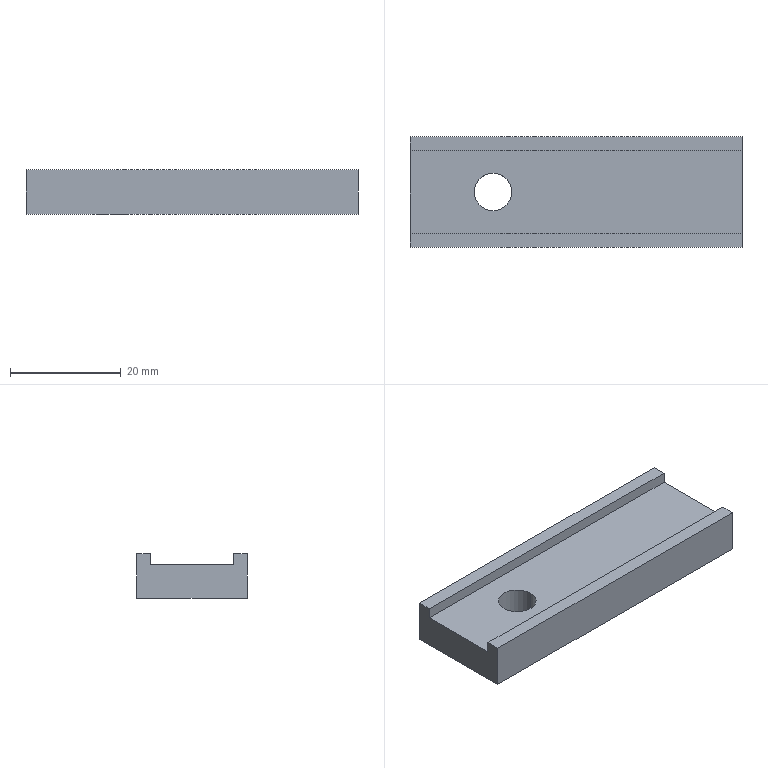Part | STEP file | Tensioning fixed block QY-1-10 | 1 solid | 12 faces | box 60 x 20 x 8 mm | volume 7582 mm3 | plane 10 | cylinder 2 | commonest cylinder face diameters 6.8 x2
STEP:
#1=CARTESIAN_POINT('',(0.,0.,0.));
#2=DIRECTION('',(0.,0.,1.));
#3=DIRECTION('',(1.,0.,0.));
#4=AXIS2_PLACEMENT_3D('',#1,#2,#3);
#5=CARTESIAN_POINT('',(-11.6,0.,0.));
#6=VERTEX_POINT('',#5);
#7=CARTESIAN_POINT('',(-11.6,0.,6.));
#8=VERTEX_POINT('',#7);
#9=CARTESIAN_POINT('',(-11.6,0.,6.));
#10=DIRECTION('',(0.,0.,1.));
#11=VECTOR('',#10,1.);
#12=LINE('',#9,#11);
#13=CARTESIAN_POINT('',(-15.,0.,6.));
#14=DIRECTION('',(0.,0.,1.));
#15=DIRECTION('',(1.,0.,0.));
#16=AXIS2_PLACEMENT_3D('',#13,#14,#15);
#17=CYLINDRICAL_SURFACE('',#16,3.4);
#18=CARTESIAN_POINT('',(6.283,0.));
#19=DIRECTION('',(0.,1.));
#20=VECTOR('',#19,1.);
#21=LINE('',#18,#20);
#22=(GEOMETRIC_REPRESENTATION_CONTEXT(2)PARAMETRIC_REPRESENTATION_CONTEXT()REPRESENTATION_CONTEXT('',''));
#23=DEFINITIONAL_REPRESENTATION('',(#21),#22);
#24=PCURVE('',#17,#23);
#25=CARTESIAN_POINT('',(-15.,0.,6.));
#26=DIRECTION('',(0.,0.,1.));
#27=DIRECTION('',(1.,0.,0.));
#28=AXIS2_PLACEMENT_3D('',#25,#26,#27);
#29=CYLINDRICAL_SURFACE('',#28,3.4);
#30=CARTESIAN_POINT('',(0.,0.));
#31=DIRECTION('',(0.,1.));
#32=VECTOR('',#31,1.);
#33=LINE('',#30,#32);
#34=(GEOMETRIC_REPRESENTATION_CONTEXT(2)PARAMETRIC_REPRESENTATION_CONTEXT()REPRESENTATION_CONTEXT('',''));
#35=DEFINITIONAL_REPRESENTATION('',(#33),#34);
#36=PCURVE('',#29,#35);
#37=SURFACE_CURVE('',#12,(#24,#36),.PCURVE_S1.);
#38=EDGE_CURVE('',#6,#8,#37,.T.);
#39=ORIENTED_EDGE('',*,*,#38,.T.);
#40=CARTESIAN_POINT('',(-18.4,0.,6.));
#41=VERTEX_POINT('',#40);
#42=CARTESIAN_POINT('',(-15.,0.,6.));
#43=DIRECTION('',(0.,0.,1.));
#44=DIRECTION('',(1.,0.,0.));
#45=AXIS2_PLACEMENT_3D('',#42,#43,#44);
#46=CIRCLE('',#45,3.4);
#47=CARTESIAN_POINT('',(0.,0.));
#48=DIRECTION('',(1.,0.));
#49=VECTOR('',#48,1.);
#50=LINE('',#47,#49);
#51=(GEOMETRIC_REPRESENTATION_CONTEXT(2)PARAMETRIC_REPRESENTATION_CONTEXT()REPRESENTATION_CONTEXT('',''));
#52=DEFINITIONAL_REPRESENTATION('',(#50),#51);
#53=PCURVE('',#17,#52);
#54=CARTESIAN_POINT('',(0.,0.,6.));
#55=DIRECTION('',(0.,0.,-1.));
#56=DIRECTION('',(-1.,0.,0.));
#57=AXIS2_PLACEMENT_3D('',#54,#55,#56);
#58=PLANE('',#57);
#59=CARTESIAN_POINT('',(11.6,0.));
#60=CARTESIAN_POINT('',(11.6,5.889));
#61=CARTESIAN_POINT('',(16.7,2.944));
#62=CARTESIAN_POINT('',(21.8,0.));
#63=CARTESIAN_POINT('',(16.7,-2.944));
#64=CARTESIAN_POINT('',(11.6,-5.889));
#65=CARTESIAN_POINT('',(11.6,0.));
#66=(BOUNDED_CURVE()B_SPLINE_CURVE(2,(#59,#60,#61,#62,#63,#64,#65),.UNSPECIFIED.,.T.,.F.)B_SPLINE_CURVE_WITH_KNOTS((1,2,2,2,2,1),(-2.094,0.,2.094,4.189,6.283,8.378),.UNSPECIFIED.)CURVE()GEOMETRIC_REPRESENTATION_ITEM()RATIONAL_B_SPLINE_CURVE((1.,0.5,1.,0.5,1.,0.5,1.))REPRESENTATION_ITEM(''));
#67=(GEOMETRIC_REPRESENTATION_CONTEXT(2)PARAMETRIC_REPRESENTATION_CONTEXT()REPRESENTATION_CONTEXT('',''));
#68=DEFINITIONAL_REPRESENTATION('',(#66),#67);
#69=PCURVE('',#58,#68);
#70=SURFACE_CURVE('',#46,(#53,#69),.PCURVE_S1.);
#71=EDGE_CURVE('',#41,#8,#70,.T.);
#72=ORIENTED_EDGE('',*,*,#71,.F.);
#73=CARTESIAN_POINT('',(-18.4,0.,0.));
#74=VERTEX_POINT('',#73);
#75=CARTESIAN_POINT('',(-18.4,0.,6.));
#76=DIRECTION('',(0.,0.,1.));
#77=VECTOR('',#76,1.);
#78=LINE('',#75,#77);
#79=CARTESIAN_POINT('',(3.142,0.));
#80=DIRECTION('',(0.,1.));
#81=VECTOR('',#80,1.);
#82=LINE('',#79,#81);
#83=(GEOMETRIC_REPRESENTATION_CONTEXT(2)PARAMETRIC_REPRESENTATION_CONTEXT()REPRESENTATION_CONTEXT('',''));
#84=DEFINITIONAL_REPRESENTATION('',(#82),#83);
#85=PCURVE('',#17,#84);
#86=CARTESIAN_POINT('',(3.142,0.));
#87=DIRECTION('',(0.,1.));
#88=VECTOR('',#87,1.);
#89=LINE('',#86,#88);
#90=(GEOMETRIC_REPRESENTATION_CONTEXT(2)PARAMETRIC_REPRESENTATION_CONTEXT()REPRESENTATION_CONTEXT('',''));
#91=DEFINITIONAL_REPRESENTATION('',(#89),#90);
#92=PCURVE('',#29,#91);
#93=SURFACE_CURVE('',#78,(#85,#92),.PCURVE_S1.);
#94=EDGE_CURVE('',#74,#41,#93,.T.);
#95=ORIENTED_EDGE('',*,*,#94,.F.);
#96=CARTESIAN_POINT('',(-15.,0.,0.));
#97=DIRECTION('',(0.,0.,1.));
#98=DIRECTION('',(1.,0.,0.));
#99=AXIS2_PLACEMENT_3D('',#96,#97,#98);
#100=CIRCLE('',#99,3.4);
#101=CARTESIAN_POINT('',(0.,-6.));
#102=DIRECTION('',(1.,0.));
#103=VECTOR('',#102,1.);
#104=LINE('',#101,#103);
#105=(GEOMETRIC_REPRESENTATION_CONTEXT(2)PARAMETRIC_REPRESENTATION_CONTEXT()REPRESENTATION_CONTEXT('',''));
#106=DEFINITIONAL_REPRESENTATION('',(#104),#105);
#107=PCURVE('',#17,#106);
#108=CARTESIAN_POINT('',(0.,0.,0.));
#109=DIRECTION('',(0.,0.,1.));
#110=DIRECTION('',(1.,0.,0.));
#111=AXIS2_PLACEMENT_3D('',#108,#109,#110);
#112=PLANE('',#111);
#113=CARTESIAN_POINT('',(-15.,0.));
#114=DIRECTION('',(1.,0.));
#115=AXIS2_PLACEMENT_2D('',#113,#114);
#116=CIRCLE('',#115,3.4);
#117=(GEOMETRIC_REPRESENTATION_CONTEXT(2)PARAMETRIC_REPRESENTATION_CONTEXT()REPRESENTATION_CONTEXT('',''));
#118=DEFINITIONAL_REPRESENTATION('',(#116),#117);
#119=PCURVE('',#112,#118);
#120=SURFACE_CURVE('',#100,(#107,#119),.PCURVE_S1.);
#121=EDGE_CURVE('',#74,#6,#120,.T.);
#122=ORIENTED_EDGE('',*,*,#121,.T.);
#123=EDGE_LOOP('',(#39,#72,#95,#122));
#124=FACE_BOUND('',#123,.F.);
#125=ADVANCED_FACE('',(#124),#17,.F.);
#126=CARTESIAN_POINT('',(-30.,-7.5,8.));
#127=VERTEX_POINT('',#126);
#128=CARTESIAN_POINT('',(30.,-7.5,8.));
#129=VERTEX_POINT('',#128);
#130=CARTESIAN_POINT('',(0.,-7.5,8.));
#131=DIRECTION('',(1.,0.,0.));
#132=VECTOR('',#131,1.);
#133=LINE('',#130,#132);
#134=CARTESIAN_POINT('',(0.,0.,8.));
#135=DIRECTION('',(0.,0.,1.));
#136=DIRECTION('',(1.,0.,0.));
#137=AXIS2_PLACEMENT_3D('',#134,#135,#136);
#138=PLANE('',#137);
#139=CARTESIAN_POINT('',(0.,-7.5));
#140=DIRECTION('',(1.,0.));
#141=VECTOR('',#140,1.);
#142=LINE('',#139,#141);
#143=(GEOMETRIC_REPRESENTATION_CONTEXT(2)PARAMETRIC_REPRESENTATION_CONTEXT()REPRESENTATION_CONTEXT('',''));
#144=DEFINITIONAL_REPRESENTATION('',(#142),#143);
#145=PCURVE('',#138,#144);
#146=CARTESIAN_POINT('',(-35.049,-7.5,6.));
#147=DIRECTION('',(0.,-1.,0.));
#148=DIRECTION('',(0.,0.,-1.));
#149=AXIS2_PLACEMENT_3D('',#146,#147,#148);
#150=PLANE('',#149);
#151=CARTESIAN_POINT('',(-2.,35.049));
#152=DIRECTION('',(0.,1.));
#153=VECTOR('',#152,1.);
#154=LINE('',#151,#153);
#155=(GEOMETRIC_REPRESENTATION_CONTEXT(2)PARAMETRIC_REPRESENTATION_CONTEXT()REPRESENTATION_CONTEXT('',''));
#156=DEFINITIONAL_REPRESENTATION('',(#154),#155);
#157=PCURVE('',#150,#156);
#158=SURFACE_CURVE('',#133,(#145,#157),.PCURVE_S1.);
#159=EDGE_CURVE('',#127,#129,#158,.T.);
#160=ORIENTED_EDGE('',*,*,#159,.F.);
#161=CARTESIAN_POINT('',(-30.,-10.,8.));
#162=VERTEX_POINT('',#161);
#163=CARTESIAN_POINT('',(-30.,10.,8.));
#164=DIRECTION('',(0.,-1.,0.));
#165=VECTOR('',#164,1.);
#166=LINE('',#163,#165);
#167=CARTESIAN_POINT('',(-30.,10.));
#168=DIRECTION('',(0.,-1.));
#169=VECTOR('',#168,1.);
#170=LINE('',#167,#169);
#171=(GEOMETRIC_REPRESENTATION_CONTEXT(2)PARAMETRIC_REPRESENTATION_CONTEXT()REPRESENTATION_CONTEXT('',''));
#172=DEFINITIONAL_REPRESENTATION('',(#170),#171);
#173=PCURVE('',#138,#172);
#174=CARTESIAN_POINT('',(-30.,10.,8.));
#175=DIRECTION('',(1.,0.,0.));
#176=DIRECTION('',(0.,1.,0.));
#177=AXIS2_PLACEMENT_3D('',#174,#175,#176);
#178=PLANE('',#177);
#179=CARTESIAN_POINT('',(0.,0.));
#180=DIRECTION('',(-1.,0.));
#181=VECTOR('',#180,1.);
#182=LINE('',#179,#181);
#183=(GEOMETRIC_REPRESENTATION_CONTEXT(2)PARAMETRIC_REPRESENTATION_CONTEXT()REPRESENTATION_CONTEXT('',''));
#184=DEFINITIONAL_REPRESENTATION('',(#182),#183);
#185=PCURVE('',#178,#184);
#186=SURFACE_CURVE('',#166,(#173,#185),.PCURVE_S1.);
#187=EDGE_CURVE('',#127,#162,#186,.T.);
#188=ORIENTED_EDGE('',*,*,#187,.T.);
#189=CARTESIAN_POINT('',(30.,-10.,8.));
#190=VERTEX_POINT('',#189);
#191=CARTESIAN_POINT('',(-30.,-10.,8.));
#192=DIRECTION('',(1.,0.,0.));
#193=VECTOR('',#192,1.);
#194=LINE('',#191,#193);
#195=CARTESIAN_POINT('',(-30.,-10.));
#196=DIRECTION('',(1.,0.));
#197=VECTOR('',#196,1.);
#198=LINE('',#195,#197);
#199=(GEOMETRIC_REPRESENTATION_CONTEXT(2)PARAMETRIC_REPRESENTATION_CONTEXT()REPRESENTATION_CONTEXT('',''));
#200=DEFINITIONAL_REPRESENTATION('',(#198),#199);
#201=PCURVE('',#138,#200);
#202=CARTESIAN_POINT('',(-30.,-10.,8.));
#203=DIRECTION('',(0.,1.,0.));
#204=DIRECTION('',(0.,0.,1.));
#205=AXIS2_PLACEMENT_3D('',#202,#203,#204);
#206=PLANE('',#205);
#207=CARTESIAN_POINT('',(0.,0.));
#208=DIRECTION('',(0.,1.));
#209=VECTOR('',#208,1.);
#210=LINE('',#207,#209);
#211=(GEOMETRIC_REPRESENTATION_CONTEXT(2)PARAMETRIC_REPRESENTATION_CONTEXT()REPRESENTATION_CONTEXT('',''));
#212=DEFINITIONAL_REPRESENTATION('',(#210),#211);
#213=PCURVE('',#206,#212);
#214=SURFACE_CURVE('',#194,(#201,#213),.PCURVE_S1.);
#215=EDGE_CURVE('',#162,#190,#214,.T.);
#216=ORIENTED_EDGE('',*,*,#215,.T.);
#217=CARTESIAN_POINT('',(30.,10.,8.));
#218=DIRECTION('',(0.,1.,0.));
#219=VECTOR('',#218,1.);
#220=LINE('',#217,#219);
#221=CARTESIAN_POINT('',(30.,10.));
#222=DIRECTION('',(0.,1.));
#223=VECTOR('',#222,1.);
#224=LINE('',#221,#223);
#225=(GEOMETRIC_REPRESENTATION_CONTEXT(2)PARAMETRIC_REPRESENTATION_CONTEXT()REPRESENTATION_CONTEXT('',''));
#226=DEFINITIONAL_REPRESENTATION('',(#224),#225);
#227=PCURVE('',#138,#226);
#228=CARTESIAN_POINT('',(30.,10.,8.));
#229=DIRECTION('',(-1.,0.,0.));
#230=DIRECTION('',(0.,-1.,0.));
#231=AXIS2_PLACEMENT_3D('',#228,#229,#230);
#232=PLANE('',#231);
#233=CARTESIAN_POINT('',(0.,0.));
#234=DIRECTION('',(-1.,0.));
#235=VECTOR('',#234,1.);
#236=LINE('',#233,#235);
#237=(GEOMETRIC_REPRESENTATION_CONTEXT(2)PARAMETRIC_REPRESENTATION_CONTEXT()REPRESENTATION_CONTEXT('',''));
#238=DEFINITIONAL_REPRESENTATION('',(#236),#237);
#239=PCURVE('',#232,#238);
#240=SURFACE_CURVE('',#220,(#227,#239),.PCURVE_S1.);
#241=EDGE_CURVE('',#190,#129,#240,.T.);
#242=ORIENTED_EDGE('',*,*,#241,.T.);
#243=EDGE_LOOP('',(#160,#188,#216,#242));
#244=FACE_BOUND('',#243,.T.);
#245=ADVANCED_FACE('',(#244),#138,.T.);
#246=CARTESIAN_POINT('',(30.,7.5,6.));
#247=VERTEX_POINT('',#246);
#248=CARTESIAN_POINT('',(30.,-7.5,6.));
#249=VERTEX_POINT('',#248);
#250=CARTESIAN_POINT('',(30.,10.,6.));
#251=DIRECTION('',(0.,-1.,0.));
#252=VECTOR('',#251,1.);
#253=LINE('',#250,#252);
#254=CARTESIAN_POINT('',(0.,-2.));
#255=DIRECTION('',(1.,0.));
#256=VECTOR('',#255,1.);
#257=LINE('',#254,#256);
#258=(GEOMETRIC_REPRESENTATION_CONTEXT(2)PARAMETRIC_REPRESENTATION_CONTEXT()REPRESENTATION_CONTEXT('',''));
#259=DEFINITIONAL_REPRESENTATION('',(#257),#258);
#260=PCURVE('',#232,#259);
#261=CARTESIAN_POINT('',(-30.,10.));
#262=DIRECTION('',(0.,-1.));
#263=VECTOR('',#262,1.);
#264=LINE('',#261,#263);
#265=(GEOMETRIC_REPRESENTATION_CONTEXT(2)PARAMETRIC_REPRESENTATION_CONTEXT()REPRESENTATION_CONTEXT('',''));
#266=DEFINITIONAL_REPRESENTATION('',(#264),#265);
#267=PCURVE('',#58,#266);
#268=SURFACE_CURVE('',#253,(#260,#267),.PCURVE_S1.);
#269=EDGE_CURVE('',#247,#249,#268,.T.);
#270=ORIENTED_EDGE('',*,*,#269,.T.);
#271=CARTESIAN_POINT('',(30.,-7.5,8.));
#272=DIRECTION('',(0.,0.,1.));
#273=VECTOR('',#272,1.);
#274=LINE('',#271,#273);
#275=CARTESIAN_POINT('',(17.5,0.));
#276=DIRECTION('',(0.,1.));
#277=VECTOR('',#276,1.);
#278=LINE('',#275,#277);
#279=(GEOMETRIC_REPRESENTATION_CONTEXT(2)PARAMETRIC_REPRESENTATION_CONTEXT()REPRESENTATION_CONTEXT('',''));
#280=DEFINITIONAL_REPRESENTATION('',(#278),#279);
#281=PCURVE('',#232,#280);
#282=CARTESIAN_POINT('',(-2.,65.049));
#283=DIRECTION('',(-1.,0.));
#284=VECTOR('',#283,1.);
#285=LINE('',#282,#284);
#286=(GEOMETRIC_REPRESENTATION_CONTEXT(2)PARAMETRIC_REPRESENTATION_CONTEXT()REPRESENTATION_CONTEXT('',''));
#287=DEFINITIONAL_REPRESENTATION('',(#285),#286);
#288=PCURVE('',#150,#287);
#289=SURFACE_CURVE('',#274,(#281,#288),.PCURVE_S1.);
#290=EDGE_CURVE('',#249,#129,#289,.T.);
#291=ORIENTED_EDGE('',*,*,#290,.T.);
#292=ORIENTED_EDGE('',*,*,#241,.F.);
#293=CARTESIAN_POINT('',(30.,-10.,0.));
#294=VERTEX_POINT('',#293);
#295=CARTESIAN_POINT('',(30.,-10.,8.));
#296=DIRECTION('',(0.,0.,-1.));
#297=VECTOR('',#296,1.);
#298=LINE('',#295,#297);
#299=CARTESIAN_POINT('',(20.,0.));
#300=DIRECTION('',(0.,-1.));
#301=VECTOR('',#300,1.);
#302=LINE('',#299,#301);
#303=(GEOMETRIC_REPRESENTATION_CONTEXT(2)PARAMETRIC_REPRESENTATION_CONTEXT()REPRESENTATION_CONTEXT('',''));
#304=DEFINITIONAL_REPRESENTATION('',(#302),#303);
#305=PCURVE('',#232,#304);
#306=CARTESIAN_POINT('',(0.,60.));
#307=DIRECTION('',(-1.,0.));
#308=VECTOR('',#307,1.);
#309=LINE('',#306,#308);
#310=(GEOMETRIC_REPRESENTATION_CONTEXT(2)PARAMETRIC_REPRESENTATION_CONTEXT()REPRESENTATION_CONTEXT('',''));
#311=DEFINITIONAL_REPRESENTATION('',(#309),#310);
#312=PCURVE('',#206,#311);
#313=SURFACE_CURVE('',#298,(#305,#312),.PCURVE_S1.);
#314=EDGE_CURVE('',#190,#294,#313,.T.);
#315=ORIENTED_EDGE('',*,*,#314,.T.);
#316=CARTESIAN_POINT('',(30.,10.,0.));
#317=VERTEX_POINT('',#316);
#318=CARTESIAN_POINT('',(30.,10.,0.));
#319=DIRECTION('',(0.,1.,0.));
#320=VECTOR('',#319,1.);
#321=LINE('',#318,#320);
#322=CARTESIAN_POINT('',(0.,-8.));
#323=DIRECTION('',(-1.,0.));
#324=VECTOR('',#323,1.);
#325=LINE('',#322,#324);
#326=(GEOMETRIC_REPRESENTATION_CONTEXT(2)PARAMETRIC_REPRESENTATION_CONTEXT()REPRESENTATION_CONTEXT('',''));
#327=DEFINITIONAL_REPRESENTATION('',(#325),#326);
#328=PCURVE('',#232,#327);
#329=CARTESIAN_POINT('',(30.,10.));
#330=DIRECTION('',(0.,1.));
#331=VECTOR('',#330,1.);
#332=LINE('',#329,#331);
#333=(GEOMETRIC_REPRESENTATION_CONTEXT(2)PARAMETRIC_REPRESENTATION_CONTEXT()REPRESENTATION_CONTEXT('',''));
#334=DEFINITIONAL_REPRESENTATION('',(#332),#333);
#335=PCURVE('',#112,#334);
#336=SURFACE_CURVE('',#321,(#328,#335),.PCURVE_S1.);
#337=EDGE_CURVE('',#294,#317,#336,.T.);
#338=ORIENTED_EDGE('',*,*,#337,.T.);
#339=CARTESIAN_POINT('',(30.,10.,8.));
#340=VERTEX_POINT('',#339);
#341=CARTESIAN_POINT('',(30.,10.,8.));
#342=DIRECTION('',(0.,0.,-1.));
#343=VECTOR('',#342,1.);
#344=LINE('',#341,#343);
#345=CARTESIAN_POINT('',(0.,0.));
#346=DIRECTION('',(0.,-1.));
#347=VECTOR('',#346,1.);
#348=LINE('',#345,#347);
#349=(GEOMETRIC_REPRESENTATION_CONTEXT(2)PARAMETRIC_REPRESENTATION_CONTEXT()REPRESENTATION_CONTEXT('',''));
#350=DEFINITIONAL_REPRESENTATION('',(#348),#349);
#351=PCURVE('',#232,#350);
#352=CARTESIAN_POINT('',(-30.,10.,8.));
#353=DIRECTION('',(0.,-1.,0.));
#354=DIRECTION('',(0.,0.,-1.));
#355=AXIS2_PLACEMENT_3D('',#352,#353,#354);
#356=PLANE('',#355);
#357=CARTESIAN_POINT('',(0.,60.));
#358=DIRECTION('',(1.,0.));
#359=VECTOR('',#358,1.);
#360=LINE('',#357,#359);
#361=(GEOMETRIC_REPRESENTATION_CONTEXT(2)PARAMETRIC_REPRESENTATION_CONTEXT()REPRESENTATION_CONTEXT('',''));
#362=DEFINITIONAL_REPRESENTATION('',(#360),#361);
#363=PCURVE('',#356,#362);
#364=SURFACE_CURVE('',#344,(#351,#363),.PCURVE_S1.);
#365=EDGE_CURVE('',#340,#317,#364,.T.);
#366=ORIENTED_EDGE('',*,*,#365,.F.);
#367=CARTESIAN_POINT('',(30.,7.5,8.));
#368=VERTEX_POINT('',#367);
#369=CARTESIAN_POINT('',(30.,10.,8.));
#370=DIRECTION('',(0.,1.,0.));
#371=VECTOR('',#370,1.);
#372=LINE('',#369,#371);
#373=CARTESIAN_POINT('',(0.,0.));
#374=DIRECTION('',(-1.,0.));
#375=VECTOR('',#374,1.);
#376=LINE('',#373,#375);
#377=(GEOMETRIC_REPRESENTATION_CONTEXT(2)PARAMETRIC_REPRESENTATION_CONTEXT()REPRESENTATION_CONTEXT('',''));
#378=DEFINITIONAL_REPRESENTATION('',(#376),#377);
#379=PCURVE('',#232,#378);
#380=CARTESIAN_POINT('',(0.,0.,8.));
#381=DIRECTION('',(0.,0.,1.));
#382=DIRECTION('',(1.,0.,0.));
#383=AXIS2_PLACEMENT_3D('',#380,#381,#382);
#384=PLANE('',#383);
#385=CARTESIAN_POINT('',(30.,10.));
#386=DIRECTION('',(0.,1.));
#387=VECTOR('',#386,1.);
#388=LINE('',#385,#387);
#389=(GEOMETRIC_REPRESENTATION_CONTEXT(2)PARAMETRIC_REPRESENTATION_CONTEXT()REPRESENTATION_CONTEXT('',''));
#390=DEFINITIONAL_REPRESENTATION('',(#388),#389);
#391=PCURVE('',#384,#390);
#392=SURFACE_CURVE('',#372,(#379,#391),.PCURVE_S1.);
#393=EDGE_CURVE('',#368,#340,#392,.T.);
#394=ORIENTED_EDGE('',*,*,#393,.F.);
#395=CARTESIAN_POINT('',(30.,7.5,8.));
#396=DIRECTION('',(0.,0.,-1.));
#397=VECTOR('',#396,1.);
#398=LINE('',#395,#397);
#399=CARTESIAN_POINT('',(2.5,0.));
#400=DIRECTION('',(0.,-1.));
#401=VECTOR('',#400,1.);
#402=LINE('',#399,#401);
#403=(GEOMETRIC_REPRESENTATION_CONTEXT(2)PARAMETRIC_REPRESENTATION_CONTEXT()REPRESENTATION_CONTEXT('',''));
#404=DEFINITIONAL_REPRESENTATION('',(#402),#403);
#405=PCURVE('',#232,#404);
#406=CARTESIAN_POINT('',(-35.049,7.5,6.));
#407=DIRECTION('',(0.,1.,0.));
#408=DIRECTION('',(0.,0.,1.));
#409=AXIS2_PLACEMENT_3D('',#406,#407,#408);
#410=PLANE('',#409);
#411=CARTESIAN_POINT('',(2.,65.049));
#412=DIRECTION('',(-1.,0.));
#413=VECTOR('',#412,1.);
#414=LINE('',#411,#413);
#415=(GEOMETRIC_REPRESENTATION_CONTEXT(2)PARAMETRIC_REPRESENTATION_CONTEXT()REPRESENTATION_CONTEXT('',''));
#416=DEFINITIONAL_REPRESENTATION('',(#414),#415);
#417=PCURVE('',#410,#416);
#418=SURFACE_CURVE('',#398,(#405,#417),.PCURVE_S1.);
#419=EDGE_CURVE('',#368,#247,#418,.T.);
#420=ORIENTED_EDGE('',*,*,#419,.T.);
#421=EDGE_LOOP('',(#270,#291,#292,#315,#338,#366,#394,#420));
#422=FACE_BOUND('',#421,.T.);
#423=ADVANCED_FACE('',(#422),#232,.F.);
#424=CARTESIAN_POINT('',(-30.,10.,0.));
#425=VERTEX_POINT('',#424);
#426=CARTESIAN_POINT('',(-30.,10.,0.));
#427=DIRECTION('',(-1.,0.,0.));
#428=VECTOR('',#427,1.);
#429=LINE('',#426,#428);
#430=CARTESIAN_POINT('',(8.,0.));
#431=DIRECTION('',(0.,-1.));
#432=VECTOR('',#431,1.);
#433=LINE('',#430,#432);
#434=(GEOMETRIC_REPRESENTATION_CONTEXT(2)PARAMETRIC_REPRESENTATION_CONTEXT()REPRESENTATION_CONTEXT('',''));
#435=DEFINITIONAL_REPRESENTATION('',(#433),#434);
#436=PCURVE('',#356,#435);
#437=CARTESIAN_POINT('',(-30.,10.));
#438=DIRECTION('',(-1.,0.));
#439=VECTOR('',#438,1.);
#440=LINE('',#437,#439);
#441=(GEOMETRIC_REPRESENTATION_CONTEXT(2)PARAMETRIC_REPRESENTATION_CONTEXT()REPRESENTATION_CONTEXT('',''));
#442=DEFINITIONAL_REPRESENTATION('',(#440),#441);
#443=PCURVE('',#112,#442);
#444=SURFACE_CURVE('',#429,(#436,#443),.PCURVE_S1.);
#445=EDGE_CURVE('',#317,#425,#444,.T.);
#446=ORIENTED_EDGE('',*,*,#445,.T.);
#447=CARTESIAN_POINT('',(-30.,10.,8.));
#448=VERTEX_POINT('',#447);
#449=CARTESIAN_POINT('',(-30.,10.,8.));
#450=DIRECTION('',(0.,0.,-1.));
#451=VECTOR('',#450,1.);
#452=LINE('',#449,#451);
#453=CARTESIAN_POINT('',(0.,0.));
#454=DIRECTION('',(1.,0.));
#455=VECTOR('',#454,1.);
#456=LINE('',#453,#455);
#457=(GEOMETRIC_REPRESENTATION_CONTEXT(2)PARAMETRIC_REPRESENTATION_CONTEXT()REPRESENTATION_CONTEXT('',''));
#458=DEFINITIONAL_REPRESENTATION('',(#456),#457);
#459=PCURVE('',#356,#458);
#460=CARTESIAN_POINT('',(0.,0.));
#461=DIRECTION('',(0.,-1.));
#462=VECTOR('',#461,1.);
#463=LINE('',#460,#462);
#464=(GEOMETRIC_REPRESENTATION_CONTEXT(2)PARAMETRIC_REPRESENTATION_CONTEXT()REPRESENTATION_CONTEXT('',''));
#465=DEFINITIONAL_REPRESENTATION('',(#463),#464);
#466=PCURVE('',#178,#465);
#467=SURFACE_CURVE('',#452,(#459,#466),.PCURVE_S1.);
#468=EDGE_CURVE('',#448,#425,#467,.T.);
#469=ORIENTED_EDGE('',*,*,#468,.F.);
#470=CARTESIAN_POINT('',(-30.,10.,8.));
#471=DIRECTION('',(-1.,0.,0.));
#472=VECTOR('',#471,1.);
#473=LINE('',#470,#472);
#474=CARTESIAN_POINT('',(0.,0.));
#475=DIRECTION('',(0.,-1.));
#476=VECTOR('',#475,1.);
#477=LINE('',#474,#476);
#478=(GEOMETRIC_REPRESENTATION_CONTEXT(2)PARAMETRIC_REPRESENTATION_CONTEXT()REPRESENTATION_CONTEXT('',''));
#479=DEFINITIONAL_REPRESENTATION('',(#477),#478);
#480=PCURVE('',#356,#479);
#481=CARTESIAN_POINT('',(-30.,10.));
#482=DIRECTION('',(-1.,0.));
#483=VECTOR('',#482,1.);
#484=LINE('',#481,#483);
#485=(GEOMETRIC_REPRESENTATION_CONTEXT(2)PARAMETRIC_REPRESENTATION_CONTEXT()REPRESENTATION_CONTEXT('',''));
#486=DEFINITIONAL_REPRESENTATION('',(#484),#485);
#487=PCURVE('',#384,#486);
#488=SURFACE_CURVE('',#473,(#480,#487),.PCURVE_S1.);
#489=EDGE_CURVE('',#340,#448,#488,.T.);
#490=ORIENTED_EDGE('',*,*,#489,.F.);
#491=ORIENTED_EDGE('',*,*,#365,.T.);
#492=EDGE_LOOP('',(#446,#469,#490,#491));
#493=FACE_BOUND('',#492,.T.);
#494=ADVANCED_FACE('',(#493),#356,.F.);
#495=ORIENTED_EDGE('',*,*,#187,.F.);
#496=CARTESIAN_POINT('',(-30.,-7.5,6.));
#497=VERTEX_POINT('',#496);
#498=CARTESIAN_POINT('',(-30.,-7.5,8.));
#499=DIRECTION('',(0.,0.,-1.));
#500=VECTOR('',#499,1.);
#501=LINE('',#498,#500);
#502=CARTESIAN_POINT('',(-17.5,0.));
#503=DIRECTION('',(0.,-1.));
#504=VECTOR('',#503,1.);
#505=LINE('',#502,#504);
#506=(GEOMETRIC_REPRESENTATION_CONTEXT(2)PARAMETRIC_REPRESENTATION_CONTEXT()REPRESENTATION_CONTEXT('',''));
#507=DEFINITIONAL_REPRESENTATION('',(#505),#506);
#508=PCURVE('',#178,#507);
#509=CARTESIAN_POINT('',(-2.,5.049));
#510=DIRECTION('',(1.,0.));
#511=VECTOR('',#510,1.);
#512=LINE('',#509,#511);
#513=(GEOMETRIC_REPRESENTATION_CONTEXT(2)PARAMETRIC_REPRESENTATION_CONTEXT()REPRESENTATION_CONTEXT('',''));
#514=DEFINITIONAL_REPRESENTATION('',(#512),#513);
#515=PCURVE('',#150,#514);
#516=SURFACE_CURVE('',#501,(#508,#515),.PCURVE_S1.);
#517=EDGE_CURVE('',#127,#497,#516,.T.);
#518=ORIENTED_EDGE('',*,*,#517,.T.);
#519=CARTESIAN_POINT('',(-30.,7.5,6.));
#520=VERTEX_POINT('',#519);
#521=CARTESIAN_POINT('',(-30.,10.,6.));
#522=DIRECTION('',(0.,1.,0.));
#523=VECTOR('',#522,1.);
#524=LINE('',#521,#523);
#525=CARTESIAN_POINT('',(0.,-2.));
#526=DIRECTION('',(1.,0.));
#527=VECTOR('',#526,1.);
#528=LINE('',#525,#527);
#529=(GEOMETRIC_REPRESENTATION_CONTEXT(2)PARAMETRIC_REPRESENTATION_CONTEXT()REPRESENTATION_CONTEXT('',''));
#530=DEFINITIONAL_REPRESENTATION('',(#528),#529);
#531=PCURVE('',#178,#530);
#532=CARTESIAN_POINT('',(30.,10.));
#533=DIRECTION('',(0.,1.));
#534=VECTOR('',#533,1.);
#535=LINE('',#532,#534);
#536=(GEOMETRIC_REPRESENTATION_CONTEXT(2)PARAMETRIC_REPRESENTATION_CONTEXT()REPRESENTATION_CONTEXT('',''));
#537=DEFINITIONAL_REPRESENTATION('',(#535),#536);
#538=PCURVE('',#58,#537);
#539=SURFACE_CURVE('',#524,(#531,#538),.PCURVE_S1.);
#540=EDGE_CURVE('',#497,#520,#539,.T.);
#541=ORIENTED_EDGE('',*,*,#540,.T.);
#542=CARTESIAN_POINT('',(-30.,7.5,8.));
#543=VERTEX_POINT('',#542);
#544=CARTESIAN_POINT('',(-30.,7.5,8.));
#545=DIRECTION('',(0.,0.,1.));
#546=VECTOR('',#545,1.);
#547=LINE('',#544,#546);
#548=CARTESIAN_POINT('',(-2.5,0.));
#549=DIRECTION('',(0.,1.));
#550=VECTOR('',#549,1.);
#551=LINE('',#548,#550);
#552=(GEOMETRIC_REPRESENTATION_CONTEXT(2)PARAMETRIC_REPRESENTATION_CONTEXT()REPRESENTATION_CONTEXT('',''));
#553=DEFINITIONAL_REPRESENTATION('',(#551),#552);
#554=PCURVE('',#178,#553);
#555=CARTESIAN_POINT('',(2.,5.049));
#556=DIRECTION('',(1.,0.));
#557=VECTOR('',#556,1.);
#558=LINE('',#555,#557);
#559=(GEOMETRIC_REPRESENTATION_CONTEXT(2)PARAMETRIC_REPRESENTATION_CONTEXT()REPRESENTATION_CONTEXT('',''));
#560=DEFINITIONAL_REPRESENTATION('',(#558),#559);
#561=PCURVE('',#410,#560);
#562=SURFACE_CURVE('',#547,(#554,#561),.PCURVE_S1.);
#563=EDGE_CURVE('',#520,#543,#562,.T.);
#564=ORIENTED_EDGE('',*,*,#563,.T.);
#565=CARTESIAN_POINT('',(-30.,10.,8.));
#566=DIRECTION('',(0.,-1.,0.));
#567=VECTOR('',#566,1.);
#568=LINE('',#565,#567);
#569=CARTESIAN_POINT('',(0.,0.));
#570=DIRECTION('',(-1.,0.));
#571=VECTOR('',#570,1.);
#572=LINE('',#569,#571);
#573=(GEOMETRIC_REPRESENTATION_CONTEXT(2)PARAMETRIC_REPRESENTATION_CONTEXT()REPRESENTATION_CONTEXT('',''));
#574=DEFINITIONAL_REPRESENTATION('',(#572),#573);
#575=PCURVE('',#178,#574);
#576=CARTESIAN_POINT('',(-30.,10.));
#577=DIRECTION('',(0.,-1.));
#578=VECTOR('',#577,1.);
#579=LINE('',#576,#578);
#580=(GEOMETRIC_REPRESENTATION_CONTEXT(2)PARAMETRIC_REPRESENTATION_CONTEXT()REPRESENTATION_CONTEXT('',''));
#581=DEFINITIONAL_REPRESENTATION('',(#579),#580);
#582=PCURVE('',#384,#581);
#583=SURFACE_CURVE('',#568,(#575,#582),.PCURVE_S1.);
#584=EDGE_CURVE('',#448,#543,#583,.T.);
#585=ORIENTED_EDGE('',*,*,#584,.F.);
#586=ORIENTED_EDGE('',*,*,#468,.T.);
#587=CARTESIAN_POINT('',(-30.,-10.,0.));
#588=VERTEX_POINT('',#587);
#589=CARTESIAN_POINT('',(-30.,10.,0.));
#590=DIRECTION('',(0.,-1.,0.));
#591=VECTOR('',#590,1.);
#592=LINE('',#589,#591);
#593=CARTESIAN_POINT('',(0.,-8.));
#594=DIRECTION('',(-1.,0.));
#595=VECTOR('',#594,1.);
#596=LINE('',#593,#595);
#597=(GEOMETRIC_REPRESENTATION_CONTEXT(2)PARAMETRIC_REPRESENTATION_CONTEXT()REPRESENTATION_CONTEXT('',''));
#598=DEFINITIONAL_REPRESENTATION('',(#596),#597);
#599=PCURVE('',#178,#598);
#600=CARTESIAN_POINT('',(-30.,10.));
#601=DIRECTION('',(0.,-1.));
#602=VECTOR('',#601,1.);
#603=LINE('',#600,#602);
#604=(GEOMETRIC_REPRESENTATION_CONTEXT(2)PARAMETRIC_REPRESENTATION_CONTEXT()REPRESENTATION_CONTEXT('',''));
#605=DEFINITIONAL_REPRESENTATION('',(#603),#604);
#606=PCURVE('',#112,#605);
#607=SURFACE_CURVE('',#592,(#599,#606),.PCURVE_S1.);
#608=EDGE_CURVE('',#425,#588,#607,.T.);
#609=ORIENTED_EDGE('',*,*,#608,.T.);
#610=CARTESIAN_POINT('',(-30.,-10.,8.));
#611=DIRECTION('',(0.,0.,-1.));
#612=VECTOR('',#611,1.);
#613=LINE('',#610,#612);
#614=CARTESIAN_POINT('',(-20.,0.));
#615=DIRECTION('',(0.,-1.));
#616=VECTOR('',#615,1.);
#617=LINE('',#614,#616);
#618=(GEOMETRIC_REPRESENTATION_CONTEXT(2)PARAMETRIC_REPRESENTATION_CONTEXT()REPRESENTATION_CONTEXT('',''));
#619=DEFINITIONAL_REPRESENTATION('',(#617),#618);
#620=PCURVE('',#178,#619);
#621=CARTESIAN_POINT('',(0.,0.));
#622=DIRECTION('',(-1.,0.));
#623=VECTOR('',#622,1.);
#624=LINE('',#621,#623);
#625=(GEOMETRIC_REPRESENTATION_CONTEXT(2)PARAMETRIC_REPRESENTATION_CONTEXT()REPRESENTATION_CONTEXT('',''));
#626=DEFINITIONAL_REPRESENTATION('',(#624),#625);
#627=PCURVE('',#206,#626);
#628=SURFACE_CURVE('',#613,(#620,#627),.PCURVE_S1.);
#629=EDGE_CURVE('',#162,#588,#628,.T.);
#630=ORIENTED_EDGE('',*,*,#629,.F.);
#631=EDGE_LOOP('',(#495,#518,#541,#564,#585,#586,#609,#630));
#632=FACE_BOUND('',#631,.T.);
#633=ADVANCED_FACE('',(#632),#178,.F.);
#634=CARTESIAN_POINT('',(-30.,-10.,0.));
#635=DIRECTION('',(1.,0.,0.));
#636=VECTOR('',#635,1.);
#637=LINE('',#634,#636);
#638=CARTESIAN_POINT('',(-8.,0.));
#639=DIRECTION('',(0.,1.));
#640=VECTOR('',#639,1.);
#641=LINE('',#638,#640);
#642=(GEOMETRIC_REPRESENTATION_CONTEXT(2)PARAMETRIC_REPRESENTATION_CONTEXT()REPRESENTATION_CONTEXT('',''));
#643=DEFINITIONAL_REPRESENTATION('',(#641),#642);
#644=PCURVE('',#206,#643);
#645=CARTESIAN_POINT('',(-30.,-10.));
#646=DIRECTION('',(1.,0.));
#647=VECTOR('',#646,1.);
#648=LINE('',#645,#647);
#649=(GEOMETRIC_REPRESENTATION_CONTEXT(2)PARAMETRIC_REPRESENTATION_CONTEXT()REPRESENTATION_CONTEXT('',''));
#650=DEFINITIONAL_REPRESENTATION('',(#648),#649);
#651=PCURVE('',#112,#650);
#652=SURFACE_CURVE('',#637,(#644,#651),.PCURVE_S1.);
#653=EDGE_CURVE('',#588,#294,#652,.T.);
#654=ORIENTED_EDGE('',*,*,#653,.T.);
#655=ORIENTED_EDGE('',*,*,#314,.F.);
#656=ORIENTED_EDGE('',*,*,#215,.F.);
#657=ORIENTED_EDGE('',*,*,#629,.T.);
#658=EDGE_LOOP('',(#654,#655,#656,#657));
#659=FACE_BOUND('',#658,.T.);
#660=ADVANCED_FACE('',(#659),#206,.F.);
#661=CARTESIAN_POINT('',(0.,7.5,8.));
#662=DIRECTION('',(-1.,0.,0.));
#663=VECTOR('',#662,1.);
#664=LINE('',#661,#663);
#665=CARTESIAN_POINT('',(0.,7.5));
#666=DIRECTION('',(-1.,0.));
#667=VECTOR('',#666,1.);
#668=LINE('',#665,#667);
#669=(GEOMETRIC_REPRESENTATION_CONTEXT(2)PARAMETRIC_REPRESENTATION_CONTEXT()REPRESENTATION_CONTEXT('',''));
#670=DEFINITIONAL_REPRESENTATION('',(#668),#669);
#671=PCURVE('',#384,#670);
#672=CARTESIAN_POINT('',(2.,35.049));
#673=DIRECTION('',(0.,-1.));
#674=VECTOR('',#673,1.);
#675=LINE('',#672,#674);
#676=(GEOMETRIC_REPRESENTATION_CONTEXT(2)PARAMETRIC_REPRESENTATION_CONTEXT()REPRESENTATION_CONTEXT('',''));
#677=DEFINITIONAL_REPRESENTATION('',(#675),#676);
#678=PCURVE('',#410,#677);
#679=SURFACE_CURVE('',#664,(#671,#678),.PCURVE_S1.);
#680=EDGE_CURVE('',#368,#543,#679,.T.);
#681=ORIENTED_EDGE('',*,*,#680,.F.);
#682=ORIENTED_EDGE('',*,*,#393,.T.);
#683=ORIENTED_EDGE('',*,*,#489,.T.);
#684=ORIENTED_EDGE('',*,*,#584,.T.);
#685=EDGE_LOOP('',(#681,#682,#683,#684));
#686=FACE_BOUND('',#685,.T.);
#687=ADVANCED_FACE('',(#686),#384,.T.);
#688=CARTESIAN_POINT('',(-15.,0.,0.));
#689=DIRECTION('',(0.,0.,1.));
#690=DIRECTION('',(1.,0.,0.));
#691=AXIS2_PLACEMENT_3D('',#688,#689,#690);
#692=CIRCLE('',#691,3.4);
#693=CARTESIAN_POINT('',(-15.,0.));
#694=DIRECTION('',(1.,0.));
#695=AXIS2_PLACEMENT_2D('',#693,#694);
#696=CIRCLE('',#695,3.4);
#697=(GEOMETRIC_REPRESENTATION_CONTEXT(2)PARAMETRIC_REPRESENTATION_CONTEXT()REPRESENTATION_CONTEXT('',''));
#698=DEFINITIONAL_REPRESENTATION('',(#696),#697);
#699=PCURVE('',#112,#698);
#700=CARTESIAN_POINT('',(0.,-6.));
#701=DIRECTION('',(1.,0.));
#702=VECTOR('',#701,1.);
#703=LINE('',#700,#702);
#704=(GEOMETRIC_REPRESENTATION_CONTEXT(2)PARAMETRIC_REPRESENTATION_CONTEXT()REPRESENTATION_CONTEXT('',''));
#705=DEFINITIONAL_REPRESENTATION('',(#703),#704);
#706=PCURVE('',#29,#705);
#707=SURFACE_CURVE('',#692,(#699,#706),.PCURVE_S1.);
#708=EDGE_CURVE('',#6,#74,#707,.T.);
#709=ORIENTED_EDGE('',*,*,#708,.T.);
#710=ORIENTED_EDGE('',*,*,#121,.T.);
#711=EDGE_LOOP('',(#709,#710));
#712=FACE_BOUND('',#711,.T.);
#713=ORIENTED_EDGE('',*,*,#337,.F.);
#714=ORIENTED_EDGE('',*,*,#653,.F.);
#715=ORIENTED_EDGE('',*,*,#608,.F.);
#716=ORIENTED_EDGE('',*,*,#445,.F.);
#717=EDGE_LOOP('',(#713,#714,#715,#716));
#718=FACE_BOUND('',#717,.T.);
#719=ADVANCED_FACE('',(#712,#718),#112,.F.);
#720=CARTESIAN_POINT('',(-15.,0.,6.));
#721=DIRECTION('',(0.,0.,1.));
#722=DIRECTION('',(1.,0.,0.));
#723=AXIS2_PLACEMENT_3D('',#720,#721,#722);
#724=CIRCLE('',#723,3.4);
#725=CARTESIAN_POINT('',(11.6,0.));
#726=CARTESIAN_POINT('',(11.6,5.889));
#727=CARTESIAN_POINT('',(16.7,2.944));
#728=CARTESIAN_POINT('',(21.8,0.));
#729=CARTESIAN_POINT('',(16.7,-2.944));
#730=CARTESIAN_POINT('',(11.6,-5.889));
#731=CARTESIAN_POINT('',(11.6,0.));
#732=(BOUNDED_CURVE()B_SPLINE_CURVE(2,(#725,#726,#727,#728,#729,#730,#731),.UNSPECIFIED.,.T.,.F.)B_SPLINE_CURVE_WITH_KNOTS((1,2,2,2,2,1),(-2.094,0.,2.094,4.189,6.283,8.378),.UNSPECIFIED.)CURVE()GEOMETRIC_REPRESENTATION_ITEM()RATIONAL_B_SPLINE_CURVE((1.,0.5,1.,0.5,1.,0.5,1.))REPRESENTATION_ITEM(''));
#733=(GEOMETRIC_REPRESENTATION_CONTEXT(2)PARAMETRIC_REPRESENTATION_CONTEXT()REPRESENTATION_CONTEXT('',''));
#734=DEFINITIONAL_REPRESENTATION('',(#732),#733);
#735=PCURVE('',#58,#734);
#736=CARTESIAN_POINT('',(0.,0.));
#737=DIRECTION('',(1.,0.));
#738=VECTOR('',#737,1.);
#739=LINE('',#736,#738);
#740=(GEOMETRIC_REPRESENTATION_CONTEXT(2)PARAMETRIC_REPRESENTATION_CONTEXT()REPRESENTATION_CONTEXT('',''));
#741=DEFINITIONAL_REPRESENTATION('',(#739),#740);
#742=PCURVE('',#29,#741);
#743=SURFACE_CURVE('',#724,(#735,#742),.PCURVE_S1.);
#744=EDGE_CURVE('',#8,#41,#743,.T.);
#745=ORIENTED_EDGE('',*,*,#744,.F.);
#746=ORIENTED_EDGE('',*,*,#71,.F.);
#747=EDGE_LOOP('',(#745,#746));
#748=FACE_BOUND('',#747,.T.);
#749=CARTESIAN_POINT('',(-35.049,7.5,6.));
#750=DIRECTION('',(-1.,0.,0.));
#751=VECTOR('',#750,1.);
#752=LINE('',#749,#751);
#753=CARTESIAN_POINT('',(35.049,7.5));
#754=DIRECTION('',(1.,0.));
#755=VECTOR('',#754,1.);
#756=LINE('',#753,#755);
#757=(GEOMETRIC_REPRESENTATION_CONTEXT(2)PARAMETRIC_REPRESENTATION_CONTEXT()REPRESENTATION_CONTEXT('',''));
#758=DEFINITIONAL_REPRESENTATION('',(#756),#757);
#759=PCURVE('',#58,#758);
#760=CARTESIAN_POINT('',(0.,0.));
#761=DIRECTION('',(0.,-1.));
#762=VECTOR('',#761,1.);
#763=LINE('',#760,#762);
#764=(GEOMETRIC_REPRESENTATION_CONTEXT(2)PARAMETRIC_REPRESENTATION_CONTEXT()REPRESENTATION_CONTEXT('',''));
#765=DEFINITIONAL_REPRESENTATION('',(#763),#764);
#766=PCURVE('',#410,#765);
#767=SURFACE_CURVE('',#752,(#759,#766),.PCURVE_S1.);
#768=EDGE_CURVE('',#247,#520,#767,.T.);
#769=ORIENTED_EDGE('',*,*,#768,.T.);
#770=ORIENTED_EDGE('',*,*,#540,.F.);
#771=CARTESIAN_POINT('',(-35.049,-7.5,6.));
#772=DIRECTION('',(1.,0.,0.));
#773=VECTOR('',#772,1.);
#774=LINE('',#771,#773);
#775=CARTESIAN_POINT('',(35.049,-7.5));
#776=DIRECTION('',(-1.,0.));
#777=VECTOR('',#776,1.);
#778=LINE('',#775,#777);
#779=(GEOMETRIC_REPRESENTATION_CONTEXT(2)PARAMETRIC_REPRESENTATION_CONTEXT()REPRESENTATION_CONTEXT('',''));
#780=DEFINITIONAL_REPRESENTATION('',(#778),#779);
#781=PCURVE('',#58,#780);
#782=CARTESIAN_POINT('',(0.,0.));
#783=DIRECTION('',(0.,1.));
#784=VECTOR('',#783,1.);
#785=LINE('',#782,#784);
#786=(GEOMETRIC_REPRESENTATION_CONTEXT(2)PARAMETRIC_REPRESENTATION_CONTEXT()REPRESENTATION_CONTEXT('',''));
#787=DEFINITIONAL_REPRESENTATION('',(#785),#786);
#788=PCURVE('',#150,#787);
#789=SURFACE_CURVE('',#774,(#781,#788),.PCURVE_S1.);
#790=EDGE_CURVE('',#497,#249,#789,.T.);
#791=ORIENTED_EDGE('',*,*,#790,.T.);
#792=ORIENTED_EDGE('',*,*,#269,.F.);
#793=EDGE_LOOP('',(#769,#770,#791,#792));
#794=FACE_BOUND('',#793,.T.);
#795=ADVANCED_FACE('',(#748,#794),#58,.F.);
#796=ORIENTED_EDGE('',*,*,#790,.F.);
#797=ORIENTED_EDGE('',*,*,#517,.F.);
#798=ORIENTED_EDGE('',*,*,#159,.T.);
#799=ORIENTED_EDGE('',*,*,#290,.F.);
#800=EDGE_LOOP('',(#796,#797,#798,#799));
#801=FACE_BOUND('',#800,.T.);
#802=ADVANCED_FACE('',(#801),#150,.F.);
#803=ORIENTED_EDGE('',*,*,#680,.T.);
#804=ORIENTED_EDGE('',*,*,#563,.F.);
#805=ORIENTED_EDGE('',*,*,#768,.F.);
#806=ORIENTED_EDGE('',*,*,#419,.F.);
#807=EDGE_LOOP('',(#803,#804,#805,#806));
#808=FACE_BOUND('',#807,.T.);
#809=ADVANCED_FACE('',(#808),#410,.F.);
#810=ORIENTED_EDGE('',*,*,#744,.F.);
#811=ORIENTED_EDGE('',*,*,#38,.F.);
#812=ORIENTED_EDGE('',*,*,#708,.T.);
#813=ORIENTED_EDGE('',*,*,#94,.T.);
#814=EDGE_LOOP('',(#810,#811,#812,#813));
#815=FACE_BOUND('',#814,.F.);
#816=ADVANCED_FACE('',(#815),#29,.F.);
#817=CLOSED_SHELL('',(#125,#245,#423,#494,#633,#660,#687,#719,#795,#802,#809,#816));
#818=MANIFOLD_SOLID_BREP('',#817);
#819=(LENGTH_UNIT()NAMED_UNIT(*)SI_UNIT(.MILLI.,.METRE.));
#820=UNCERTAINTY_MEASURE_WITH_UNIT(LENGTH_MEASURE(0.0000001),#819,'','');
#821=(NAMED_UNIT(*)PLANE_ANGLE_UNIT()SI_UNIT($,.RADIAN.));
#822=(NAMED_UNIT(*)SI_UNIT($,.STERADIAN.)SOLID_ANGLE_UNIT());
#823=(GEOMETRIC_REPRESENTATION_CONTEXT(3)GLOBAL_UNCERTAINTY_ASSIGNED_CONTEXT((#820))GLOBAL_UNIT_ASSIGNED_CONTEXT((#819,#821,#822))REPRESENTATION_CONTEXT('',''));
#824=ADVANCED_BREP_SHAPE_REPRESENTATION('',(#4,#818),#823);